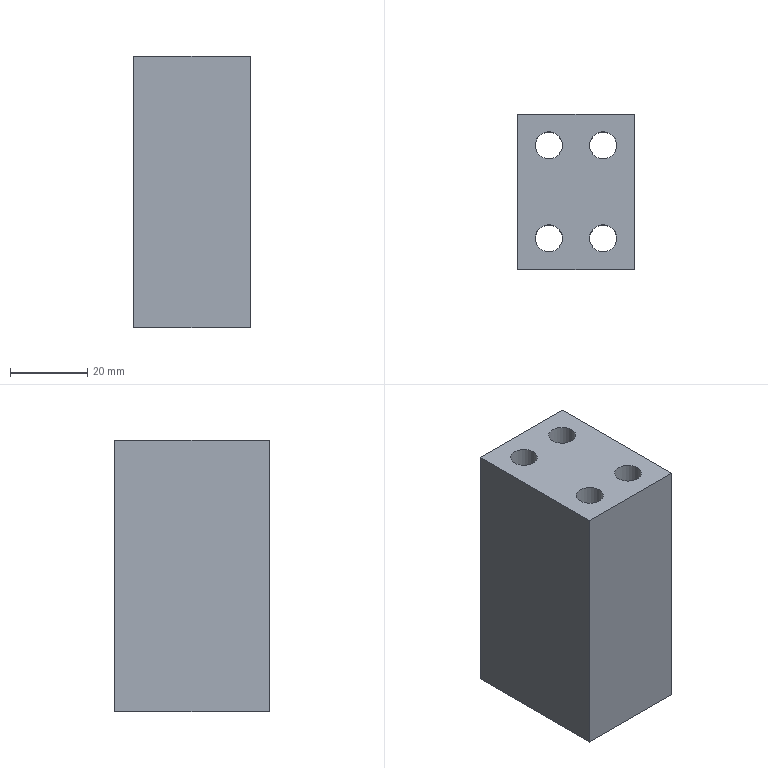Part | NX | features LB-19 2 | 1 solid | 10 faces | box 30 x 40 x 70 mm | volume 73197 mm3 | plane 6 | cylinder 4 | commonest cylinder face diameters 7.009 x4
STEP:
#1=CARTESIAN_POINT('',(4417.594,-693.122,803.716));
#2=VERTEX_POINT('',#1);
#3=CARTESIAN_POINT('',(4417.594,-693.122,873.716));
#4=VERTEX_POINT('',#3);
#5=CARTESIAN_POINT('',(4417.594,-693.122,833.029));
#6=DIRECTION('',(0.,0.,1.));
#7=VECTOR('',#6,1000.);
#8=LINE('',#5,#7);
#9=EDGE_CURVE('',#2,#4,#8,.T.);
#10=ORIENTED_EDGE('',*,*,#9,.F.);
#11=CARTESIAN_POINT('',(4387.594,-693.122,803.716));
#12=VERTEX_POINT('',#11);
#13=CARTESIAN_POINT('',(4402.594,-693.122,803.716));
#14=DIRECTION('',(-1.,0.,0.));
#15=VECTOR('',#14,1000.);
#16=LINE('',#13,#15);
#17=EDGE_CURVE('',#12,#2,#16,.F.);
#18=ORIENTED_EDGE('',*,*,#17,.F.);
#19=CARTESIAN_POINT('',(4387.594,-693.122,873.716));
#20=VERTEX_POINT('',#19);
#21=CARTESIAN_POINT('',(4387.594,-693.122,833.029));
#22=DIRECTION('',(0.,0.,-1.));
#23=VECTOR('',#22,1000.);
#24=LINE('',#21,#23);
#25=EDGE_CURVE('',#20,#12,#24,.T.);
#26=ORIENTED_EDGE('',*,*,#25,.F.);
#27=CARTESIAN_POINT('',(3639.721,-693.122,873.716));
#28=DIRECTION('',(-1.,0.,0.));
#29=VECTOR('',#28,1000.);
#30=LINE('',#27,#29);
#31=EDGE_CURVE('',#4,#20,#30,.T.);
#32=ORIENTED_EDGE('',*,*,#31,.F.);
#33=EDGE_LOOP('',(#10,#18,#26,#32));
#34=FACE_BOUND('',#33,.T.);
#35=CARTESIAN_POINT('',(4402.594,-693.122,833.029));
#36=DIRECTION('',(0.,-1.,0.));
#37=DIRECTION('',(0.,0.,-1.));
#38=AXIS2_PLACEMENT_3D('',#35,#36,#37);
#39=PLANE('',#38);
#40=ADVANCED_FACE('',(#34),#39,.F.);
#41=CARTESIAN_POINT('',(4387.594,-733.122,803.716));
#42=VERTEX_POINT('',#41);
#43=CARTESIAN_POINT('',(4387.594,-813.596,803.716));
#44=DIRECTION('',(0.,1.,0.));
#45=VECTOR('',#44,1000.);
#46=LINE('',#43,#45);
#47=EDGE_CURVE('',#12,#42,#46,.F.);
#48=ORIENTED_EDGE('',*,*,#47,.T.);
#49=CARTESIAN_POINT('',(4387.594,-733.122,873.716));
#50=VERTEX_POINT('',#49);
#51=CARTESIAN_POINT('',(4387.594,-733.122,868.343));
#52=DIRECTION('',(0.,0.,1.));
#53=VECTOR('',#52,1000.);
#54=LINE('',#51,#53);
#55=EDGE_CURVE('',#42,#50,#54,.T.);
#56=ORIENTED_EDGE('',*,*,#55,.T.);
#57=CARTESIAN_POINT('',(4387.594,-813.596,873.716));
#58=DIRECTION('',(0.,-1.,0.));
#59=VECTOR('',#58,1000.);
#60=LINE('',#57,#59);
#61=EDGE_CURVE('',#20,#50,#60,.T.);
#62=ORIENTED_EDGE('',*,*,#61,.F.);
#63=ORIENTED_EDGE('',*,*,#25,.T.);
#64=EDGE_LOOP('',(#48,#56,#62,#63));
#65=FACE_BOUND('',#64,.T.);
#66=CARTESIAN_POINT('',(4387.594,-813.596,868.343));
#67=DIRECTION('',(-1.,0.,0.));
#68=DIRECTION('',(0.,0.,-1.));
#69=AXIS2_PLACEMENT_3D('',#66,#67,#68);
#70=PLANE('',#69);
#71=ADVANCED_FACE('',(#65),#70,.T.);
#72=CARTESIAN_POINT('',(4417.594,-733.122,803.716));
#73=VERTEX_POINT('',#72);
#74=CARTESIAN_POINT('',(4417.594,-813.596,803.716));
#75=DIRECTION('',(0.,-1.,0.));
#76=VECTOR('',#75,1000.);
#77=LINE('',#74,#76);
#78=EDGE_CURVE('',#2,#73,#77,.T.);
#79=ORIENTED_EDGE('',*,*,#78,.F.);
#80=ORIENTED_EDGE('',*,*,#9,.T.);
#81=CARTESIAN_POINT('',(4417.594,-733.122,873.716));
#82=VERTEX_POINT('',#81);
#83=CARTESIAN_POINT('',(4417.594,-829.122,873.716));
#84=DIRECTION('',(0.,-1.,0.));
#85=VECTOR('',#84,1000.);
#86=LINE('',#83,#85);
#87=EDGE_CURVE('',#4,#82,#86,.T.);
#88=ORIENTED_EDGE('',*,*,#87,.T.);
#89=CARTESIAN_POINT('',(4417.594,-733.122,868.343));
#90=DIRECTION('',(0.,0.,-1.));
#91=VECTOR('',#90,1000.);
#92=LINE('',#89,#91);
#93=EDGE_CURVE('',#82,#73,#92,.T.);
#94=ORIENTED_EDGE('',*,*,#93,.T.);
#95=EDGE_LOOP('',(#79,#80,#88,#94));
#96=FACE_BOUND('',#95,.T.);
#97=CARTESIAN_POINT('',(4417.594,-813.596,868.343));
#98=DIRECTION('',(1.,0.,0.));
#99=DIRECTION('',(0.,0.,1.));
#100=AXIS2_PLACEMENT_3D('',#97,#98,#99);
#101=PLANE('',#100);
#102=ADVANCED_FACE('',(#96),#101,.T.);
#103=ORIENTED_EDGE('',*,*,#55,.F.);
#104=CARTESIAN_POINT('',(4402.594,-733.122,803.716));
#105=DIRECTION('',(1.,0.,0.));
#106=VECTOR('',#105,1000.);
#107=LINE('',#104,#106);
#108=EDGE_CURVE('',#73,#42,#107,.F.);
#109=ORIENTED_EDGE('',*,*,#108,.F.);
#110=ORIENTED_EDGE('',*,*,#93,.F.);
#111=CARTESIAN_POINT('',(3639.721,-733.122,873.716));
#112=DIRECTION('',(1.,0.,0.));
#113=VECTOR('',#112,1000.);
#114=LINE('',#111,#113);
#115=EDGE_CURVE('',#50,#82,#114,.T.);
#116=ORIENTED_EDGE('',*,*,#115,.F.);
#117=EDGE_LOOP('',(#103,#109,#110,#116));
#118=FACE_BOUND('',#117,.T.);
#119=CARTESIAN_POINT('',(4402.594,-733.122,872.029));
#120=DIRECTION('',(0.,1.,0.));
#121=DIRECTION('',(0.,0.,1.));
#122=AXIS2_PLACEMENT_3D('',#119,#120,#121);
#123=PLANE('',#122);
#124=ADVANCED_FACE('',(#118),#123,.F.);
#125=CARTESIAN_POINT('',(4399.098,-701.122,803.716));
#126=VERTEX_POINT('',#125);
#127=CARTESIAN_POINT('',(4395.594,-701.122,803.716));
#128=DIRECTION('',(0.,0.,1.));
#129=DIRECTION('',(1.,0.,0.));
#130=AXIS2_PLACEMENT_3D('',#127,#128,#129);
#131=CIRCLE('',#130,3.505);
#132=EDGE_CURVE('',#126,#126,#131,.T.);
#133=ORIENTED_EDGE('',*,*,#132,.F.);
#134=EDGE_LOOP('',(#133));
#135=FACE_BOUND('',#134,.T.);
#136=CARTESIAN_POINT('',(4399.098,-701.122,873.716));
#137=VERTEX_POINT('',#136);
#138=CARTESIAN_POINT('',(4395.594,-701.122,873.716));
#139=DIRECTION('',(0.,0.,1.));
#140=DIRECTION('',(1.,0.,0.));
#141=AXIS2_PLACEMENT_3D('',#138,#139,#140);
#142=CIRCLE('',#141,3.505);
#143=EDGE_CURVE('',#137,#137,#142,.F.);
#144=ORIENTED_EDGE('',*,*,#143,.F.);
#145=EDGE_LOOP('',(#144));
#146=FACE_BOUND('',#145,.T.);
#147=CARTESIAN_POINT('',(4395.594,-701.122,873.716));
#148=DIRECTION('',(0.,0.,-1.));
#149=DIRECTION('',(1.,0.,0.));
#150=AXIS2_PLACEMENT_3D('',#147,#148,#149);
#151=CYLINDRICAL_SURFACE('',#150,3.505);
#152=ADVANCED_FACE('',(#135,#146),#151,.F.);
#153=CARTESIAN_POINT('',(4413.098,-725.122,803.716));
#154=VERTEX_POINT('',#153);
#155=CARTESIAN_POINT('',(4409.594,-725.122,803.716));
#156=DIRECTION('',(0.,0.,1.));
#157=DIRECTION('',(1.,0.,0.));
#158=AXIS2_PLACEMENT_3D('',#155,#156,#157);
#159=CIRCLE('',#158,3.505);
#160=EDGE_CURVE('',#154,#154,#159,.T.);
#161=ORIENTED_EDGE('',*,*,#160,.F.);
#162=EDGE_LOOP('',(#161));
#163=FACE_BOUND('',#162,.T.);
#164=CARTESIAN_POINT('',(4413.098,-725.122,873.716));
#165=VERTEX_POINT('',#164);
#166=CARTESIAN_POINT('',(4409.594,-725.122,873.716));
#167=DIRECTION('',(0.,0.,1.));
#168=DIRECTION('',(1.,0.,0.));
#169=AXIS2_PLACEMENT_3D('',#166,#167,#168);
#170=CIRCLE('',#169,3.505);
#171=EDGE_CURVE('',#165,#165,#170,.F.);
#172=ORIENTED_EDGE('',*,*,#171,.F.);
#173=EDGE_LOOP('',(#172));
#174=FACE_BOUND('',#173,.T.);
#175=CARTESIAN_POINT('',(4409.594,-725.122,873.716));
#176=DIRECTION('',(0.,0.,-1.));
#177=DIRECTION('',(1.,0.,0.));
#178=AXIS2_PLACEMENT_3D('',#175,#176,#177);
#179=CYLINDRICAL_SURFACE('',#178,3.505);
#180=ADVANCED_FACE('',(#163,#174),#179,.F.);
#181=CARTESIAN_POINT('',(4413.098,-701.122,803.716));
#182=VERTEX_POINT('',#181);
#183=CARTESIAN_POINT('',(4409.594,-701.122,803.716));
#184=DIRECTION('',(0.,0.,1.));
#185=DIRECTION('',(1.,0.,0.));
#186=AXIS2_PLACEMENT_3D('',#183,#184,#185);
#187=CIRCLE('',#186,3.505);
#188=EDGE_CURVE('',#182,#182,#187,.F.);
#189=ORIENTED_EDGE('',*,*,#188,.T.);
#190=EDGE_LOOP('',(#189));
#191=FACE_BOUND('',#190,.T.);
#192=CARTESIAN_POINT('',(4413.098,-701.122,873.716));
#193=VERTEX_POINT('',#192);
#194=CARTESIAN_POINT('',(4409.594,-701.122,873.716));
#195=DIRECTION('',(0.,0.,1.));
#196=DIRECTION('',(1.,0.,0.));
#197=AXIS2_PLACEMENT_3D('',#194,#195,#196);
#198=CIRCLE('',#197,3.505);
#199=EDGE_CURVE('',#193,#193,#198,.F.);
#200=ORIENTED_EDGE('',*,*,#199,.F.);
#201=EDGE_LOOP('',(#200));
#202=FACE_BOUND('',#201,.T.);
#203=CARTESIAN_POINT('',(4409.594,-701.122,873.716));
#204=DIRECTION('',(0.,0.,-1.));
#205=DIRECTION('',(1.,0.,0.));
#206=AXIS2_PLACEMENT_3D('',#203,#204,#205);
#207=CYLINDRICAL_SURFACE('',#206,3.505);
#208=ADVANCED_FACE('',(#191,#202),#207,.F.);
#209=CARTESIAN_POINT('',(4399.098,-725.122,873.716));
#210=VERTEX_POINT('',#209);
#211=CARTESIAN_POINT('',(4395.594,-725.122,873.716));
#212=DIRECTION('',(0.,0.,1.));
#213=DIRECTION('',(1.,0.,0.));
#214=AXIS2_PLACEMENT_3D('',#211,#212,#213);
#215=CIRCLE('',#214,3.505);
#216=EDGE_CURVE('',#210,#210,#215,.F.);
#217=ORIENTED_EDGE('',*,*,#216,.T.);
#218=EDGE_LOOP('',(#217));
#219=FACE_BOUND('',#218,.T.);
#220=ORIENTED_EDGE('',*,*,#199,.T.);
#221=EDGE_LOOP('',(#220));
#222=FACE_BOUND('',#221,.T.);
#223=ORIENTED_EDGE('',*,*,#171,.T.);
#224=EDGE_LOOP('',(#223));
#225=FACE_BOUND('',#224,.T.);
#226=ORIENTED_EDGE('',*,*,#143,.T.);
#227=EDGE_LOOP('',(#226));
#228=FACE_BOUND('',#227,.T.);
#229=ORIENTED_EDGE('',*,*,#87,.F.);
#230=ORIENTED_EDGE('',*,*,#31,.T.);
#231=ORIENTED_EDGE('',*,*,#61,.T.);
#232=ORIENTED_EDGE('',*,*,#115,.T.);
#233=EDGE_LOOP('',(#229,#230,#231,#232));
#234=FACE_BOUND('',#233,.T.);
#235=CARTESIAN_POINT('',(3639.721,-829.122,873.716));
#236=DIRECTION('',(0.,0.,1.));
#237=DIRECTION('',(1.,0.,0.));
#238=AXIS2_PLACEMENT_3D('',#235,#236,#237);
#239=PLANE('',#238);
#240=ADVANCED_FACE('',(#219,#222,#225,#228,#234),#239,.T.);
#241=CARTESIAN_POINT('',(4399.098,-725.122,803.716));
#242=VERTEX_POINT('',#241);
#243=CARTESIAN_POINT('',(4395.594,-725.122,803.716));
#244=DIRECTION('',(0.,0.,1.));
#245=DIRECTION('',(1.,0.,0.));
#246=AXIS2_PLACEMENT_3D('',#243,#244,#245);
#247=CIRCLE('',#246,3.505);
#248=EDGE_CURVE('',#242,#242,#247,.F.);
#249=ORIENTED_EDGE('',*,*,#248,.T.);
#250=EDGE_LOOP('',(#249));
#251=FACE_BOUND('',#250,.T.);
#252=ORIENTED_EDGE('',*,*,#216,.F.);
#253=EDGE_LOOP('',(#252));
#254=FACE_BOUND('',#253,.T.);
#255=CARTESIAN_POINT('',(4395.594,-725.122,873.716));
#256=DIRECTION('',(0.,0.,-1.));
#257=DIRECTION('',(1.,0.,0.));
#258=AXIS2_PLACEMENT_3D('',#255,#256,#257);
#259=CYLINDRICAL_SURFACE('',#258,3.505);
#260=ADVANCED_FACE('',(#251,#254),#259,.F.);
#261=ORIENTED_EDGE('',*,*,#132,.T.);
#262=EDGE_LOOP('',(#261));
#263=FACE_BOUND('',#262,.T.);
#264=ORIENTED_EDGE('',*,*,#188,.F.);
#265=EDGE_LOOP('',(#264));
#266=FACE_BOUND('',#265,.T.);
#267=ORIENTED_EDGE('',*,*,#248,.F.);
#268=EDGE_LOOP('',(#267));
#269=FACE_BOUND('',#268,.T.);
#270=ORIENTED_EDGE('',*,*,#160,.T.);
#271=EDGE_LOOP('',(#270));
#272=FACE_BOUND('',#271,.T.);
#273=ORIENTED_EDGE('',*,*,#47,.F.);
#274=ORIENTED_EDGE('',*,*,#17,.T.);
#275=ORIENTED_EDGE('',*,*,#78,.T.);
#276=ORIENTED_EDGE('',*,*,#108,.T.);
#277=EDGE_LOOP('',(#273,#274,#275,#276));
#278=FACE_BOUND('',#277,.T.);
#279=CARTESIAN_POINT('',(3317.594,-849.122,803.716));
#280=DIRECTION('',(0.,0.,1.));
#281=DIRECTION('',(1.,0.,0.));
#282=AXIS2_PLACEMENT_3D('',#279,#280,#281);
#283=PLANE('',#282);
#284=ADVANCED_FACE('',(#263,#266,#269,#272,#278),#283,.F.);
#285=CLOSED_SHELL('',(#40,#71,#102,#124,#152,#180,#208,#240,#260,#284));
#286=MANIFOLD_SOLID_BREP('',#285);
#287=(LENGTH_UNIT()NAMED_UNIT(*)SI_UNIT(.MILLI.,.METRE.));
#288=UNCERTAINTY_MEASURE_WITH_UNIT(LENGTH_MEASURE(0.00001),#287,'','');
#289=(NAMED_UNIT(*)PLANE_ANGLE_UNIT()SI_UNIT($,.RADIAN.));
#290=(NAMED_UNIT(*)SI_UNIT($,.STERADIAN.)SOLID_ANGLE_UNIT());
#291=(GEOMETRIC_REPRESENTATION_CONTEXT(3)GLOBAL_UNCERTAINTY_ASSIGNED_CONTEXT((#288))GLOBAL_UNIT_ASSIGNED_CONTEXT((#287,#289,#290))REPRESENTATION_CONTEXT('',''));
#292=ADVANCED_BREP_SHAPE_REPRESENTATION('',(#286),#291);